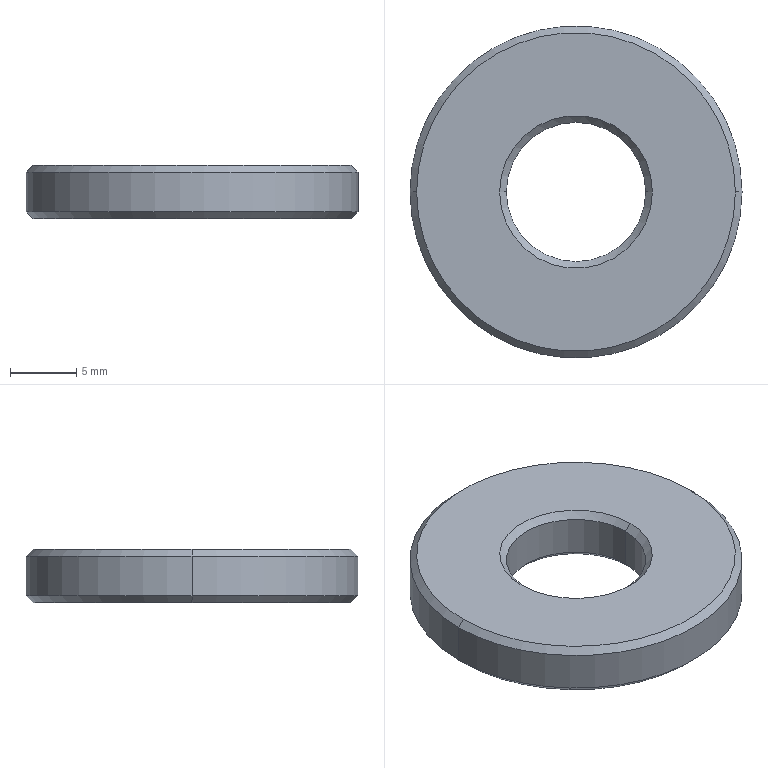Part | STEP file | PN_0101 Mount electronic clip clamp screw | 1 solid | 14 faces | box 25 x 25 x 4 mm | volume 1589 mm3 | cone 8 | cylinder 4 | plane 2 | commonest cylinder face diameters 10.5 x2 25 x2
STEP:
#1=CARTESIAN_POINT('',(0.,0.,0.));
#2=DIRECTION('',(0.,0.,1.));
#3=DIRECTION('',(1.,0.,0.));
#4=AXIS2_PLACEMENT_3D('',#1,#2,#3);
#5=CARTESIAN_POINT('',(12.,0.,4.));
#6=VERTEX_POINT('',#5);
#7=CARTESIAN_POINT('',(-12.,0.,4.));
#8=VERTEX_POINT('',#7);
#9=CARTESIAN_POINT('',(0.,0.,4.));
#10=DIRECTION('',(0.,0.,1.));
#11=DIRECTION('',(1.,0.,0.));
#12=AXIS2_PLACEMENT_3D('',#9,#10,#11);
#13=CIRCLE('',#12,12.);
#14=CARTESIAN_POINT('',(0.,0.,4.));
#15=DIRECTION('',(0.,0.,-1.));
#16=DIRECTION('',(-1.,0.,0.));
#17=AXIS2_PLACEMENT_3D('',#14,#15,#16);
#18=CONICAL_SURFACE('',#17,12.,0.7854);
#19=CARTESIAN_POINT('',(3.142,0.));
#20=DIRECTION('',(-1.,0.));
#21=VECTOR('',#20,1.);
#22=LINE('',#19,#21);
#23=(GEOMETRIC_REPRESENTATION_CONTEXT(2)PARAMETRIC_REPRESENTATION_CONTEXT()REPRESENTATION_CONTEXT('',''));
#24=DEFINITIONAL_REPRESENTATION('',(#22),#23);
#25=PCURVE('',#18,#24);
#26=CARTESIAN_POINT('',(0.,0.,4.));
#27=DIRECTION('',(0.,0.,1.));
#28=DIRECTION('',(1.,0.,0.));
#29=AXIS2_PLACEMENT_3D('',#26,#27,#28);
#30=PLANE('',#29);
#31=CARTESIAN_POINT('',(0.,0.));
#32=DIRECTION('',(1.,0.));
#33=AXIS2_PLACEMENT_2D('',#31,#32);
#34=CIRCLE('',#33,12.);
#35=(GEOMETRIC_REPRESENTATION_CONTEXT(2)PARAMETRIC_REPRESENTATION_CONTEXT()REPRESENTATION_CONTEXT('',''));
#36=DEFINITIONAL_REPRESENTATION('',(#34),#35);
#37=PCURVE('',#30,#36);
#38=SURFACE_CURVE('',#13,(#25,#37),.PCURVE_S1.);
#39=EDGE_CURVE('',#6,#8,#38,.T.);
#40=ORIENTED_EDGE('',*,*,#39,.F.);
#41=CARTESIAN_POINT('',(12.5,0.,3.5));
#42=VERTEX_POINT('',#41);
#43=CARTESIAN_POINT('',(12.,0.,4.));
#44=DIRECTION('',(0.7071,0.,-0.7071));
#45=VECTOR('',#44,1.);
#46=LINE('',#43,#45);
#47=CARTESIAN_POINT('',(3.142,0.));
#48=DIRECTION('',(0.,1.));
#49=VECTOR('',#48,1.);
#50=LINE('',#47,#49);
#51=(GEOMETRIC_REPRESENTATION_CONTEXT(2)PARAMETRIC_REPRESENTATION_CONTEXT()REPRESENTATION_CONTEXT('',''));
#52=DEFINITIONAL_REPRESENTATION('',(#50),#51);
#53=PCURVE('',#18,#52);
#54=CARTESIAN_POINT('',(0.,0.,4.));
#55=DIRECTION('',(0.,0.,-1.));
#56=DIRECTION('',(-1.,0.,0.));
#57=AXIS2_PLACEMENT_3D('',#54,#55,#56);
#58=CONICAL_SURFACE('',#57,12.,0.7854);
#59=CARTESIAN_POINT('',(3.142,0.));
#60=DIRECTION('',(0.,1.));
#61=VECTOR('',#60,1.);
#62=LINE('',#59,#61);
#63=(GEOMETRIC_REPRESENTATION_CONTEXT(2)PARAMETRIC_REPRESENTATION_CONTEXT()REPRESENTATION_CONTEXT('',''));
#64=DEFINITIONAL_REPRESENTATION('',(#62),#63);
#65=PCURVE('',#58,#64);
#66=SURFACE_CURVE('',#46,(#53,#65),.PCURVE_S1.);
#67=EDGE_CURVE('',#6,#42,#66,.T.);
#68=ORIENTED_EDGE('',*,*,#67,.T.);
#69=CARTESIAN_POINT('',(-12.5,0.,3.5));
#70=VERTEX_POINT('',#69);
#71=CARTESIAN_POINT('',(0.,0.,3.5));
#72=DIRECTION('',(0.,0.,-1.));
#73=DIRECTION('',(1.,0.,0.));
#74=AXIS2_PLACEMENT_3D('',#71,#72,#73);
#75=CIRCLE('',#74,12.5);
#76=CARTESIAN_POINT('',(-3.142,0.5));
#77=DIRECTION('',(1.,0.));
#78=VECTOR('',#77,1.);
#79=LINE('',#76,#78);
#80=(GEOMETRIC_REPRESENTATION_CONTEXT(2)PARAMETRIC_REPRESENTATION_CONTEXT()REPRESENTATION_CONTEXT('',''));
#81=DEFINITIONAL_REPRESENTATION('',(#79),#80);
#82=PCURVE('',#18,#81);
#83=CARTESIAN_POINT('',(0.,0.,4.));
#84=DIRECTION('',(0.,0.,-1.));
#85=DIRECTION('',(-1.,0.,0.));
#86=AXIS2_PLACEMENT_3D('',#83,#84,#85);
#87=CYLINDRICAL_SURFACE('',#86,12.5);
#88=CARTESIAN_POINT('',(-3.142,0.5));
#89=DIRECTION('',(1.,0.));
#90=VECTOR('',#89,1.);
#91=LINE('',#88,#90);
#92=(GEOMETRIC_REPRESENTATION_CONTEXT(2)PARAMETRIC_REPRESENTATION_CONTEXT()REPRESENTATION_CONTEXT('',''));
#93=DEFINITIONAL_REPRESENTATION('',(#91),#92);
#94=PCURVE('',#87,#93);
#95=SURFACE_CURVE('',#75,(#82,#94),.PCURVE_S1.);
#96=EDGE_CURVE('',#70,#42,#95,.T.);
#97=ORIENTED_EDGE('',*,*,#96,.F.);
#98=CARTESIAN_POINT('',(-12.,0.,4.));
#99=DIRECTION('',(-0.7071,0.,-0.7071));
#100=VECTOR('',#99,1.);
#101=LINE('',#98,#100);
#102=CARTESIAN_POINT('',(0.,0.));
#103=DIRECTION('',(0.,1.));
#104=VECTOR('',#103,1.);
#105=LINE('',#102,#104);
#106=(GEOMETRIC_REPRESENTATION_CONTEXT(2)PARAMETRIC_REPRESENTATION_CONTEXT()REPRESENTATION_CONTEXT('',''));
#107=DEFINITIONAL_REPRESENTATION('',(#105),#106);
#108=PCURVE('',#18,#107);
#109=CARTESIAN_POINT('',(6.283,0.));
#110=DIRECTION('',(0.,1.));
#111=VECTOR('',#110,1.);
#112=LINE('',#109,#111);
#113=(GEOMETRIC_REPRESENTATION_CONTEXT(2)PARAMETRIC_REPRESENTATION_CONTEXT()REPRESENTATION_CONTEXT('',''));
#114=DEFINITIONAL_REPRESENTATION('',(#112),#113);
#115=PCURVE('',#58,#114);
#116=SURFACE_CURVE('',#101,(#108,#115),.PCURVE_S1.);
#117=EDGE_CURVE('',#8,#70,#116,.T.);
#118=ORIENTED_EDGE('',*,*,#117,.F.);
#119=EDGE_LOOP('',(#40,#68,#97,#118));
#120=FACE_BOUND('',#119,.T.);
#121=ADVANCED_FACE('',(#120),#18,.T.);
#122=CARTESIAN_POINT('',(-12.,0.,0.));
#123=VERTEX_POINT('',#122);
#124=CARTESIAN_POINT('',(12.,0.,0.));
#125=VERTEX_POINT('',#124);
#126=CARTESIAN_POINT('',(0.,0.,0.));
#127=DIRECTION('',(0.,0.,-1.));
#128=DIRECTION('',(1.,0.,0.));
#129=AXIS2_PLACEMENT_3D('',#126,#127,#128);
#130=CIRCLE('',#129,12.);
#131=CARTESIAN_POINT('',(0.,0.,0.5));
#132=DIRECTION('',(0.,0.,1.));
#133=DIRECTION('',(1.,0.,0.));
#134=AXIS2_PLACEMENT_3D('',#131,#132,#133);
#135=CONICAL_SURFACE('',#134,12.5,0.7854);
#136=CARTESIAN_POINT('',(6.283,-0.5));
#137=DIRECTION('',(-1.,0.));
#138=VECTOR('',#137,1.);
#139=LINE('',#136,#138);
#140=(GEOMETRIC_REPRESENTATION_CONTEXT(2)PARAMETRIC_REPRESENTATION_CONTEXT()REPRESENTATION_CONTEXT('',''));
#141=DEFINITIONAL_REPRESENTATION('',(#139),#140);
#142=PCURVE('',#135,#141);
#143=CARTESIAN_POINT('',(0.,0.,0.));
#144=DIRECTION('',(0.,0.,1.));
#145=DIRECTION('',(1.,0.,0.));
#146=AXIS2_PLACEMENT_3D('',#143,#144,#145);
#147=PLANE('',#146);
#148=CARTESIAN_POINT('',(12.,0.));
#149=CARTESIAN_POINT('',(12.,-20.785));
#150=CARTESIAN_POINT('',(-6.,-10.392));
#151=CARTESIAN_POINT('',(-24.,0.));
#152=CARTESIAN_POINT('',(-6.,10.392));
#153=CARTESIAN_POINT('',(12.,20.785));
#154=CARTESIAN_POINT('',(12.,0.));
#155=(BOUNDED_CURVE()B_SPLINE_CURVE(2,(#148,#149,#150,#151,#152,#153,#154),.UNSPECIFIED.,.T.,.F.)B_SPLINE_CURVE_WITH_KNOTS((1,2,2,2,2,1),(-2.094,0.,2.094,4.189,6.283,8.378),.UNSPECIFIED.)CURVE()GEOMETRIC_REPRESENTATION_ITEM()RATIONAL_B_SPLINE_CURVE((1.,0.5,1.,0.5,1.,0.5,1.))REPRESENTATION_ITEM(''));
#156=(GEOMETRIC_REPRESENTATION_CONTEXT(2)PARAMETRIC_REPRESENTATION_CONTEXT()REPRESENTATION_CONTEXT('',''));
#157=DEFINITIONAL_REPRESENTATION('',(#155),#156);
#158=PCURVE('',#147,#157);
#159=SURFACE_CURVE('',#130,(#142,#158),.PCURVE_S1.);
#160=EDGE_CURVE('',#123,#125,#159,.T.);
#161=ORIENTED_EDGE('',*,*,#160,.F.);
#162=CARTESIAN_POINT('',(-12.5,0.,0.5));
#163=VERTEX_POINT('',#162);
#164=CARTESIAN_POINT('',(-12.5,0.,0.5));
#165=DIRECTION('',(-0.7071,0.,0.7071));
#166=VECTOR('',#165,1.);
#167=LINE('',#164,#166);
#168=CARTESIAN_POINT('',(3.142,0.));
#169=DIRECTION('',(0.,1.));
#170=VECTOR('',#169,1.);
#171=LINE('',#168,#170);
#172=(GEOMETRIC_REPRESENTATION_CONTEXT(2)PARAMETRIC_REPRESENTATION_CONTEXT()REPRESENTATION_CONTEXT('',''));
#173=DEFINITIONAL_REPRESENTATION('',(#171),#172);
#174=PCURVE('',#135,#173);
#175=CARTESIAN_POINT('',(0.,0.,0.5));
#176=DIRECTION('',(0.,0.,1.));
#177=DIRECTION('',(1.,0.,0.));
#178=AXIS2_PLACEMENT_3D('',#175,#176,#177);
#179=CONICAL_SURFACE('',#178,12.5,0.7854);
#180=CARTESIAN_POINT('',(3.142,0.));
#181=DIRECTION('',(0.,1.));
#182=VECTOR('',#181,1.);
#183=LINE('',#180,#182);
#184=(GEOMETRIC_REPRESENTATION_CONTEXT(2)PARAMETRIC_REPRESENTATION_CONTEXT()REPRESENTATION_CONTEXT('',''));
#185=DEFINITIONAL_REPRESENTATION('',(#183),#184);
#186=PCURVE('',#179,#185);
#187=SURFACE_CURVE('',#167,(#174,#186),.PCURVE_S1.);
#188=EDGE_CURVE('',#123,#163,#187,.T.);
#189=ORIENTED_EDGE('',*,*,#188,.T.);
#190=CARTESIAN_POINT('',(12.5,0.,0.5));
#191=VERTEX_POINT('',#190);
#192=CARTESIAN_POINT('',(0.,0.,0.5));
#193=DIRECTION('',(0.,0.,1.));
#194=DIRECTION('',(1.,0.,0.));
#195=AXIS2_PLACEMENT_3D('',#192,#193,#194);
#196=CIRCLE('',#195,12.5);
#197=CARTESIAN_POINT('',(0.,0.));
#198=DIRECTION('',(1.,0.));
#199=VECTOR('',#198,1.);
#200=LINE('',#197,#199);
#201=(GEOMETRIC_REPRESENTATION_CONTEXT(2)PARAMETRIC_REPRESENTATION_CONTEXT()REPRESENTATION_CONTEXT('',''));
#202=DEFINITIONAL_REPRESENTATION('',(#200),#201);
#203=PCURVE('',#135,#202);
#204=CARTESIAN_POINT('',(3.142,3.5));
#205=DIRECTION('',(-1.,0.));
#206=VECTOR('',#205,1.);
#207=LINE('',#204,#206);
#208=(GEOMETRIC_REPRESENTATION_CONTEXT(2)PARAMETRIC_REPRESENTATION_CONTEXT()REPRESENTATION_CONTEXT('',''));
#209=DEFINITIONAL_REPRESENTATION('',(#207),#208);
#210=PCURVE('',#87,#209);
#211=SURFACE_CURVE('',#196,(#203,#210),.PCURVE_S1.);
#212=EDGE_CURVE('',#191,#163,#211,.T.);
#213=ORIENTED_EDGE('',*,*,#212,.F.);
#214=CARTESIAN_POINT('',(12.5,0.,0.5));
#215=DIRECTION('',(0.7071,0.,0.7071));
#216=VECTOR('',#215,1.);
#217=LINE('',#214,#216);
#218=CARTESIAN_POINT('',(0.,0.));
#219=DIRECTION('',(0.,1.));
#220=VECTOR('',#219,1.);
#221=LINE('',#218,#220);
#222=(GEOMETRIC_REPRESENTATION_CONTEXT(2)PARAMETRIC_REPRESENTATION_CONTEXT()REPRESENTATION_CONTEXT('',''));
#223=DEFINITIONAL_REPRESENTATION('',(#221),#222);
#224=PCURVE('',#135,#223);
#225=CARTESIAN_POINT('',(6.283,0.));
#226=DIRECTION('',(0.,1.));
#227=VECTOR('',#226,1.);
#228=LINE('',#225,#227);
#229=(GEOMETRIC_REPRESENTATION_CONTEXT(2)PARAMETRIC_REPRESENTATION_CONTEXT()REPRESENTATION_CONTEXT('',''));
#230=DEFINITIONAL_REPRESENTATION('',(#228),#229);
#231=PCURVE('',#179,#230);
#232=SURFACE_CURVE('',#217,(#224,#231),.PCURVE_S1.);
#233=EDGE_CURVE('',#125,#191,#232,.T.);
#234=ORIENTED_EDGE('',*,*,#233,.F.);
#235=EDGE_LOOP('',(#161,#189,#213,#234));
#236=FACE_BOUND('',#235,.T.);
#237=ADVANCED_FACE('',(#236),#135,.T.);
#238=CARTESIAN_POINT('',(-5.25,0.,0.5));
#239=VERTEX_POINT('',#238);
#240=CARTESIAN_POINT('',(-5.75,0.,0.));
#241=VERTEX_POINT('',#240);
#242=CARTESIAN_POINT('',(-5.75,0.,0.));
#243=DIRECTION('',(-0.7071,0.,-0.7071));
#244=VECTOR('',#243,1.);
#245=LINE('',#242,#244);
#246=CARTESIAN_POINT('',(0.,0.,0.));
#247=DIRECTION('',(0.,0.,-1.));
#248=DIRECTION('',(-1.,0.,0.));
#249=AXIS2_PLACEMENT_3D('',#246,#247,#248);
#250=CONICAL_SURFACE('',#249,5.75,0.7854);
#251=CARTESIAN_POINT('',(6.283,0.));
#252=DIRECTION('',(0.,1.));
#253=VECTOR('',#252,1.);
#254=LINE('',#251,#253);
#255=(GEOMETRIC_REPRESENTATION_CONTEXT(2)PARAMETRIC_REPRESENTATION_CONTEXT()REPRESENTATION_CONTEXT('',''));
#256=DEFINITIONAL_REPRESENTATION('',(#254),#255);
#257=PCURVE('',#250,#256);
#258=CARTESIAN_POINT('',(0.,0.,0.));
#259=DIRECTION('',(0.,0.,-1.));
#260=DIRECTION('',(-1.,0.,0.));
#261=AXIS2_PLACEMENT_3D('',#258,#259,#260);
#262=CONICAL_SURFACE('',#261,5.75,0.7854);
#263=CARTESIAN_POINT('',(0.,0.));
#264=DIRECTION('',(0.,1.));
#265=VECTOR('',#264,1.);
#266=LINE('',#263,#265);
#267=(GEOMETRIC_REPRESENTATION_CONTEXT(2)PARAMETRIC_REPRESENTATION_CONTEXT()REPRESENTATION_CONTEXT('',''));
#268=DEFINITIONAL_REPRESENTATION('',(#266),#267);
#269=PCURVE('',#262,#268);
#270=SURFACE_CURVE('',#245,(#257,#269),.PCURVE_S1.);
#271=EDGE_CURVE('',#239,#241,#270,.T.);
#272=ORIENTED_EDGE('',*,*,#271,.T.);
#273=CARTESIAN_POINT('',(5.75,0.,0.));
#274=VERTEX_POINT('',#273);
#275=CARTESIAN_POINT('',(0.,0.,0.));
#276=DIRECTION('',(0.,0.,1.));
#277=DIRECTION('',(1.,0.,0.));
#278=AXIS2_PLACEMENT_3D('',#275,#276,#277);
#279=CIRCLE('',#278,5.75);
#280=CARTESIAN_POINT('',(9.425,0.));
#281=DIRECTION('',(-1.,0.));
#282=VECTOR('',#281,1.);
#283=LINE('',#280,#282);
#284=(GEOMETRIC_REPRESENTATION_CONTEXT(2)PARAMETRIC_REPRESENTATION_CONTEXT()REPRESENTATION_CONTEXT('',''));
#285=DEFINITIONAL_REPRESENTATION('',(#283),#284);
#286=PCURVE('',#250,#285);
#287=CARTESIAN_POINT('',(0.,0.));
#288=DIRECTION('',(1.,0.));
#289=AXIS2_PLACEMENT_2D('',#287,#288);
#290=CIRCLE('',#289,5.75);
#291=(GEOMETRIC_REPRESENTATION_CONTEXT(2)PARAMETRIC_REPRESENTATION_CONTEXT()REPRESENTATION_CONTEXT('',''));
#292=DEFINITIONAL_REPRESENTATION('',(#290),#291);
#293=PCURVE('',#147,#292);
#294=SURFACE_CURVE('',#279,(#286,#293),.PCURVE_S1.);
#295=EDGE_CURVE('',#241,#274,#294,.T.);
#296=ORIENTED_EDGE('',*,*,#295,.T.);
#297=CARTESIAN_POINT('',(5.25,0.,0.5));
#298=VERTEX_POINT('',#297);
#299=CARTESIAN_POINT('',(5.75,0.,0.));
#300=DIRECTION('',(0.7071,0.,-0.7071));
#301=VECTOR('',#300,1.);
#302=LINE('',#299,#301);
#303=CARTESIAN_POINT('',(3.142,0.));
#304=DIRECTION('',(0.,1.));
#305=VECTOR('',#304,1.);
#306=LINE('',#303,#305);
#307=(GEOMETRIC_REPRESENTATION_CONTEXT(2)PARAMETRIC_REPRESENTATION_CONTEXT()REPRESENTATION_CONTEXT('',''));
#308=DEFINITIONAL_REPRESENTATION('',(#306),#307);
#309=PCURVE('',#250,#308);
#310=CARTESIAN_POINT('',(3.142,0.));
#311=DIRECTION('',(0.,1.));
#312=VECTOR('',#311,1.);
#313=LINE('',#310,#312);
#314=(GEOMETRIC_REPRESENTATION_CONTEXT(2)PARAMETRIC_REPRESENTATION_CONTEXT()REPRESENTATION_CONTEXT('',''));
#315=DEFINITIONAL_REPRESENTATION('',(#313),#314);
#316=PCURVE('',#262,#315);
#317=SURFACE_CURVE('',#302,(#309,#316),.PCURVE_S1.);
#318=EDGE_CURVE('',#298,#274,#317,.T.);
#319=ORIENTED_EDGE('',*,*,#318,.F.);
#320=CARTESIAN_POINT('',(0.,0.,0.5));
#321=DIRECTION('',(0.,0.,-1.));
#322=DIRECTION('',(1.,0.,0.));
#323=AXIS2_PLACEMENT_3D('',#320,#321,#322);
#324=CIRCLE('',#323,5.25);
#325=CARTESIAN_POINT('',(3.142,-0.5));
#326=DIRECTION('',(1.,0.));
#327=VECTOR('',#326,1.);
#328=LINE('',#325,#327);
#329=(GEOMETRIC_REPRESENTATION_CONTEXT(2)PARAMETRIC_REPRESENTATION_CONTEXT()REPRESENTATION_CONTEXT('',''));
#330=DEFINITIONAL_REPRESENTATION('',(#328),#329);
#331=PCURVE('',#250,#330);
#332=CARTESIAN_POINT('',(0.,0.,0.));
#333=DIRECTION('',(0.,0.,1.));
#334=DIRECTION('',(1.,0.,0.));
#335=AXIS2_PLACEMENT_3D('',#332,#333,#334);
#336=CYLINDRICAL_SURFACE('',#335,5.25);
#337=CARTESIAN_POINT('',(6.283,0.5));
#338=DIRECTION('',(-1.,0.));
#339=VECTOR('',#338,1.);
#340=LINE('',#337,#339);
#341=(GEOMETRIC_REPRESENTATION_CONTEXT(2)PARAMETRIC_REPRESENTATION_CONTEXT()REPRESENTATION_CONTEXT('',''));
#342=DEFINITIONAL_REPRESENTATION('',(#340),#341);
#343=PCURVE('',#336,#342);
#344=SURFACE_CURVE('',#324,(#331,#343),.PCURVE_S1.);
#345=EDGE_CURVE('',#298,#239,#344,.T.);
#346=ORIENTED_EDGE('',*,*,#345,.T.);
#347=EDGE_LOOP('',(#272,#296,#319,#346));
#348=FACE_BOUND('',#347,.F.);
#349=ADVANCED_FACE('',(#348),#250,.F.);
#350=CARTESIAN_POINT('',(5.25,0.,3.5));
#351=VERTEX_POINT('',#350);
#352=CARTESIAN_POINT('',(5.75,0.,4.));
#353=VERTEX_POINT('',#352);
#354=CARTESIAN_POINT('',(5.25,0.,3.5));
#355=DIRECTION('',(0.7071,0.,0.7071));
#356=VECTOR('',#355,1.);
#357=LINE('',#354,#356);
#358=CARTESIAN_POINT('',(0.,0.,3.5));
#359=DIRECTION('',(0.,0.,1.));
#360=DIRECTION('',(1.,0.,0.));
#361=AXIS2_PLACEMENT_3D('',#358,#359,#360);
#362=CONICAL_SURFACE('',#361,5.25,0.7854);
#363=CARTESIAN_POINT('',(6.283,0.));
#364=DIRECTION('',(0.,1.));
#365=VECTOR('',#364,1.);
#366=LINE('',#363,#365);
#367=(GEOMETRIC_REPRESENTATION_CONTEXT(2)PARAMETRIC_REPRESENTATION_CONTEXT()REPRESENTATION_CONTEXT('',''));
#368=DEFINITIONAL_REPRESENTATION('',(#366),#367);
#369=PCURVE('',#362,#368);
#370=CARTESIAN_POINT('',(0.,0.,3.5));
#371=DIRECTION('',(0.,0.,1.));
#372=DIRECTION('',(1.,0.,0.));
#373=AXIS2_PLACEMENT_3D('',#370,#371,#372);
#374=CONICAL_SURFACE('',#373,5.25,0.7854);
#375=CARTESIAN_POINT('',(0.,0.));
#376=DIRECTION('',(0.,1.));
#377=VECTOR('',#376,1.);
#378=LINE('',#375,#377);
#379=(GEOMETRIC_REPRESENTATION_CONTEXT(2)PARAMETRIC_REPRESENTATION_CONTEXT()REPRESENTATION_CONTEXT('',''));
#380=DEFINITIONAL_REPRESENTATION('',(#378),#379);
#381=PCURVE('',#374,#380);
#382=SURFACE_CURVE('',#357,(#369,#381),.PCURVE_S1.);
#383=EDGE_CURVE('',#351,#353,#382,.T.);
#384=ORIENTED_EDGE('',*,*,#383,.T.);
#385=CARTESIAN_POINT('',(-5.75,0.,4.));
#386=VERTEX_POINT('',#385);
#387=CARTESIAN_POINT('',(0.,0.,4.));
#388=DIRECTION('',(0.,0.,-1.));
#389=DIRECTION('',(1.,0.,0.));
#390=AXIS2_PLACEMENT_3D('',#387,#388,#389);
#391=CIRCLE('',#390,5.75);
#392=CARTESIAN_POINT('',(6.283,0.5));
#393=DIRECTION('',(-1.,0.));
#394=VECTOR('',#393,1.);
#395=LINE('',#392,#394);
#396=(GEOMETRIC_REPRESENTATION_CONTEXT(2)PARAMETRIC_REPRESENTATION_CONTEXT()REPRESENTATION_CONTEXT('',''));
#397=DEFINITIONAL_REPRESENTATION('',(#395),#396);
#398=PCURVE('',#362,#397);
#399=CARTESIAN_POINT('',(5.75,0.));
#400=CARTESIAN_POINT('',(5.75,-9.959));
#401=CARTESIAN_POINT('',(-2.875,-4.98));
#402=CARTESIAN_POINT('',(-11.5,0.));
#403=CARTESIAN_POINT('',(-2.875,4.98));
#404=CARTESIAN_POINT('',(5.75,9.959));
#405=CARTESIAN_POINT('',(5.75,0.));
#406=(BOUNDED_CURVE()B_SPLINE_CURVE(2,(#399,#400,#401,#402,#403,#404,#405),.UNSPECIFIED.,.T.,.F.)B_SPLINE_CURVE_WITH_KNOTS((1,2,2,2,2,1),(-2.094,0.,2.094,4.189,6.283,8.378),.UNSPECIFIED.)CURVE()GEOMETRIC_REPRESENTATION_ITEM()RATIONAL_B_SPLINE_CURVE((1.,0.5,1.,0.5,1.,0.5,1.))REPRESENTATION_ITEM(''));
#407=(GEOMETRIC_REPRESENTATION_CONTEXT(2)PARAMETRIC_REPRESENTATION_CONTEXT()REPRESENTATION_CONTEXT('',''));
#408=DEFINITIONAL_REPRESENTATION('',(#406),#407);
#409=PCURVE('',#30,#408);
#410=SURFACE_CURVE('',#391,(#398,#409),.PCURVE_S1.);
#411=EDGE_CURVE('',#353,#386,#410,.T.);
#412=ORIENTED_EDGE('',*,*,#411,.T.);
#413=CARTESIAN_POINT('',(-5.25,0.,3.5));
#414=VERTEX_POINT('',#413);
#415=CARTESIAN_POINT('',(-5.25,0.,3.5));
#416=DIRECTION('',(-0.7071,0.,0.7071));
#417=VECTOR('',#416,1.);
#418=LINE('',#415,#417);
#419=CARTESIAN_POINT('',(3.142,0.));
#420=DIRECTION('',(0.,1.));
#421=VECTOR('',#420,1.);
#422=LINE('',#419,#421);
#423=(GEOMETRIC_REPRESENTATION_CONTEXT(2)PARAMETRIC_REPRESENTATION_CONTEXT()REPRESENTATION_CONTEXT('',''));
#424=DEFINITIONAL_REPRESENTATION('',(#422),#423);
#425=PCURVE('',#362,#424);
#426=CARTESIAN_POINT('',(3.142,0.));
#427=DIRECTION('',(0.,1.));
#428=VECTOR('',#427,1.);
#429=LINE('',#426,#428);
#430=(GEOMETRIC_REPRESENTATION_CONTEXT(2)PARAMETRIC_REPRESENTATION_CONTEXT()REPRESENTATION_CONTEXT('',''));
#431=DEFINITIONAL_REPRESENTATION('',(#429),#430);
#432=PCURVE('',#374,#431);
#433=SURFACE_CURVE('',#418,(#425,#432),.PCURVE_S1.);
#434=EDGE_CURVE('',#414,#386,#433,.T.);
#435=ORIENTED_EDGE('',*,*,#434,.F.);
#436=CARTESIAN_POINT('',(0.,0.,3.5));
#437=DIRECTION('',(0.,0.,1.));
#438=DIRECTION('',(1.,0.,0.));
#439=AXIS2_PLACEMENT_3D('',#436,#437,#438);
#440=CIRCLE('',#439,5.25);
#441=CARTESIAN_POINT('',(0.,0.));
#442=DIRECTION('',(1.,0.));
#443=VECTOR('',#442,1.);
#444=LINE('',#441,#443);
#445=(GEOMETRIC_REPRESENTATION_CONTEXT(2)PARAMETRIC_REPRESENTATION_CONTEXT()REPRESENTATION_CONTEXT('',''));
#446=DEFINITIONAL_REPRESENTATION('',(#444),#445);
#447=PCURVE('',#362,#446);
#448=CARTESIAN_POINT('',(0.,3.5));
#449=DIRECTION('',(1.,0.));
#450=VECTOR('',#449,1.);
#451=LINE('',#448,#450);
#452=(GEOMETRIC_REPRESENTATION_CONTEXT(2)PARAMETRIC_REPRESENTATION_CONTEXT()REPRESENTATION_CONTEXT('',''));
#453=DEFINITIONAL_REPRESENTATION('',(#451),#452);
#454=PCURVE('',#336,#453);
#455=SURFACE_CURVE('',#440,(#447,#454),.PCURVE_S1.);
#456=EDGE_CURVE('',#414,#351,#455,.T.);
#457=ORIENTED_EDGE('',*,*,#456,.T.);
#458=EDGE_LOOP('',(#384,#412,#435,#457));
#459=FACE_BOUND('',#458,.F.);
#460=ADVANCED_FACE('',(#459),#362,.F.);
#461=CARTESIAN_POINT('',(5.25,0.,0.));
#462=DIRECTION('',(0.,0.,1.));
#463=VECTOR('',#462,1.);
#464=LINE('',#461,#463);
#465=CARTESIAN_POINT('',(6.283,0.));
#466=DIRECTION('',(0.,1.));
#467=VECTOR('',#466,1.);
#468=LINE('',#465,#467);
#469=(GEOMETRIC_REPRESENTATION_CONTEXT(2)PARAMETRIC_REPRESENTATION_CONTEXT()REPRESENTATION_CONTEXT('',''));
#470=DEFINITIONAL_REPRESENTATION('',(#468),#469);
#471=PCURVE('',#336,#470);
#472=CARTESIAN_POINT('',(0.,0.,0.));
#473=DIRECTION('',(0.,0.,1.));
#474=DIRECTION('',(1.,0.,0.));
#475=AXIS2_PLACEMENT_3D('',#472,#473,#474);
#476=CYLINDRICAL_SURFACE('',#475,5.25);
#477=CARTESIAN_POINT('',(0.,0.));
#478=DIRECTION('',(0.,1.));
#479=VECTOR('',#478,1.);
#480=LINE('',#477,#479);
#481=(GEOMETRIC_REPRESENTATION_CONTEXT(2)PARAMETRIC_REPRESENTATION_CONTEXT()REPRESENTATION_CONTEXT('',''));
#482=DEFINITIONAL_REPRESENTATION('',(#480),#481);
#483=PCURVE('',#476,#482);
#484=SURFACE_CURVE('',#464,(#471,#483),.PCURVE_S1.);
#485=EDGE_CURVE('',#298,#351,#484,.T.);
#486=ORIENTED_EDGE('',*,*,#485,.T.);
#487=ORIENTED_EDGE('',*,*,#456,.F.);
#488=CARTESIAN_POINT('',(-5.25,0.,0.));
#489=DIRECTION('',(0.,0.,1.));
#490=VECTOR('',#489,1.);
#491=LINE('',#488,#490);
#492=CARTESIAN_POINT('',(3.142,0.));
#493=DIRECTION('',(0.,1.));
#494=VECTOR('',#493,1.);
#495=LINE('',#492,#494);
#496=(GEOMETRIC_REPRESENTATION_CONTEXT(2)PARAMETRIC_REPRESENTATION_CONTEXT()REPRESENTATION_CONTEXT('',''));
#497=DEFINITIONAL_REPRESENTATION('',(#495),#496);
#498=PCURVE('',#336,#497);
#499=CARTESIAN_POINT('',(3.142,0.));
#500=DIRECTION('',(0.,1.));
#501=VECTOR('',#500,1.);
#502=LINE('',#499,#501);
#503=(GEOMETRIC_REPRESENTATION_CONTEXT(2)PARAMETRIC_REPRESENTATION_CONTEXT()REPRESENTATION_CONTEXT('',''));
#504=DEFINITIONAL_REPRESENTATION('',(#502),#503);
#505=PCURVE('',#476,#504);
#506=SURFACE_CURVE('',#491,(#498,#505),.PCURVE_S1.);
#507=EDGE_CURVE('',#239,#414,#506,.T.);
#508=ORIENTED_EDGE('',*,*,#507,.F.);
#509=ORIENTED_EDGE('',*,*,#345,.F.);
#510=EDGE_LOOP('',(#486,#487,#508,#509));
#511=FACE_BOUND('',#510,.F.);
#512=ADVANCED_FACE('',(#511),#336,.F.);
#513=ORIENTED_EDGE('',*,*,#96,.T.);
#514=CARTESIAN_POINT('',(12.5,0.,4.));
#515=DIRECTION('',(0.,0.,-1.));
#516=VECTOR('',#515,1.);
#517=LINE('',#514,#516);
#518=CARTESIAN_POINT('',(3.142,0.));
#519=DIRECTION('',(0.,1.));
#520=VECTOR('',#519,1.);
#521=LINE('',#518,#520);
#522=(GEOMETRIC_REPRESENTATION_CONTEXT(2)PARAMETRIC_REPRESENTATION_CONTEXT()REPRESENTATION_CONTEXT('',''));
#523=DEFINITIONAL_REPRESENTATION('',(#521),#522);
#524=PCURVE('',#87,#523);
#525=CARTESIAN_POINT('',(0.,0.,4.));
#526=DIRECTION('',(0.,0.,-1.));
#527=DIRECTION('',(-1.,0.,0.));
#528=AXIS2_PLACEMENT_3D('',#525,#526,#527);
#529=CYLINDRICAL_SURFACE('',#528,12.5);
#530=CARTESIAN_POINT('',(3.142,0.));
#531=DIRECTION('',(0.,1.));
#532=VECTOR('',#531,1.);
#533=LINE('',#530,#532);
#534=(GEOMETRIC_REPRESENTATION_CONTEXT(2)PARAMETRIC_REPRESENTATION_CONTEXT()REPRESENTATION_CONTEXT('',''));
#535=DEFINITIONAL_REPRESENTATION('',(#533),#534);
#536=PCURVE('',#529,#535);
#537=SURFACE_CURVE('',#517,(#524,#536),.PCURVE_S1.);
#538=EDGE_CURVE('',#42,#191,#537,.T.);
#539=ORIENTED_EDGE('',*,*,#538,.T.);
#540=ORIENTED_EDGE('',*,*,#212,.T.);
#541=CARTESIAN_POINT('',(-12.5,0.,4.));
#542=DIRECTION('',(0.,0.,-1.));
#543=VECTOR('',#542,1.);
#544=LINE('',#541,#543);
#545=CARTESIAN_POINT('',(0.,0.));
#546=DIRECTION('',(0.,1.));
#547=VECTOR('',#546,1.);
#548=LINE('',#545,#547);
#549=(GEOMETRIC_REPRESENTATION_CONTEXT(2)PARAMETRIC_REPRESENTATION_CONTEXT()REPRESENTATION_CONTEXT('',''));
#550=DEFINITIONAL_REPRESENTATION('',(#548),#549);
#551=PCURVE('',#87,#550);
#552=CARTESIAN_POINT('',(6.283,0.));
#553=DIRECTION('',(0.,1.));
#554=VECTOR('',#553,1.);
#555=LINE('',#552,#554);
#556=(GEOMETRIC_REPRESENTATION_CONTEXT(2)PARAMETRIC_REPRESENTATION_CONTEXT()REPRESENTATION_CONTEXT('',''));
#557=DEFINITIONAL_REPRESENTATION('',(#555),#556);
#558=PCURVE('',#529,#557);
#559=SURFACE_CURVE('',#544,(#551,#558),.PCURVE_S1.);
#560=EDGE_CURVE('',#70,#163,#559,.T.);
#561=ORIENTED_EDGE('',*,*,#560,.F.);
#562=EDGE_LOOP('',(#513,#539,#540,#561));
#563=FACE_BOUND('',#562,.T.);
#564=ADVANCED_FACE('',(#563),#87,.T.);
#565=ORIENTED_EDGE('',*,*,#538,.F.);
#566=CARTESIAN_POINT('',(0.,0.,3.5));
#567=DIRECTION('',(0.,0.,-1.));
#568=DIRECTION('',(1.,0.,0.));
#569=AXIS2_PLACEMENT_3D('',#566,#567,#568);
#570=CIRCLE('',#569,12.5);
#571=CARTESIAN_POINT('',(3.142,0.5));
#572=DIRECTION('',(1.,0.));
#573=VECTOR('',#572,1.);
#574=LINE('',#571,#573);
#575=(GEOMETRIC_REPRESENTATION_CONTEXT(2)PARAMETRIC_REPRESENTATION_CONTEXT()REPRESENTATION_CONTEXT('',''));
#576=DEFINITIONAL_REPRESENTATION('',(#574),#575);
#577=PCURVE('',#529,#576);
#578=CARTESIAN_POINT('',(3.142,0.5));
#579=DIRECTION('',(1.,0.));
#580=VECTOR('',#579,1.);
#581=LINE('',#578,#580);
#582=(GEOMETRIC_REPRESENTATION_CONTEXT(2)PARAMETRIC_REPRESENTATION_CONTEXT()REPRESENTATION_CONTEXT('',''));
#583=DEFINITIONAL_REPRESENTATION('',(#581),#582);
#584=PCURVE('',#58,#583);
#585=SURFACE_CURVE('',#570,(#577,#584),.PCURVE_S1.);
#586=EDGE_CURVE('',#42,#70,#585,.T.);
#587=ORIENTED_EDGE('',*,*,#586,.T.);
#588=ORIENTED_EDGE('',*,*,#560,.T.);
#589=CARTESIAN_POINT('',(0.,0.,0.5));
#590=DIRECTION('',(0.,0.,1.));
#591=DIRECTION('',(1.,0.,0.));
#592=AXIS2_PLACEMENT_3D('',#589,#590,#591);
#593=CIRCLE('',#592,12.5);
#594=CARTESIAN_POINT('',(9.425,3.5));
#595=DIRECTION('',(-1.,0.));
#596=VECTOR('',#595,1.);
#597=LINE('',#594,#596);
#598=(GEOMETRIC_REPRESENTATION_CONTEXT(2)PARAMETRIC_REPRESENTATION_CONTEXT()REPRESENTATION_CONTEXT('',''));
#599=DEFINITIONAL_REPRESENTATION('',(#597),#598);
#600=PCURVE('',#529,#599);
#601=CARTESIAN_POINT('',(0.,0.));
#602=DIRECTION('',(1.,0.));
#603=VECTOR('',#602,1.);
#604=LINE('',#601,#603);
#605=(GEOMETRIC_REPRESENTATION_CONTEXT(2)PARAMETRIC_REPRESENTATION_CONTEXT()REPRESENTATION_CONTEXT('',''));
#606=DEFINITIONAL_REPRESENTATION('',(#604),#605);
#607=PCURVE('',#179,#606);
#608=SURFACE_CURVE('',#593,(#600,#607),.PCURVE_S1.);
#609=EDGE_CURVE('',#163,#191,#608,.T.);
#610=ORIENTED_EDGE('',*,*,#609,.T.);
#611=EDGE_LOOP('',(#565,#587,#588,#610));
#612=FACE_BOUND('',#611,.T.);
#613=ADVANCED_FACE('',(#612),#529,.T.);
#614=ORIENTED_EDGE('',*,*,#411,.T.);
#615=CARTESIAN_POINT('',(0.,0.,4.));
#616=DIRECTION('',(0.,0.,-1.));
#617=DIRECTION('',(1.,0.,0.));
#618=AXIS2_PLACEMENT_3D('',#615,#616,#617);
#619=CIRCLE('',#618,5.75);
#620=CARTESIAN_POINT('',(5.75,0.));
#621=CARTESIAN_POINT('',(5.75,-9.959));
#622=CARTESIAN_POINT('',(-2.875,-4.98));
#623=CARTESIAN_POINT('',(-11.5,0.));
#624=CARTESIAN_POINT('',(-2.875,4.98));
#625=CARTESIAN_POINT('',(5.75,9.959));
#626=CARTESIAN_POINT('',(5.75,0.));
#627=(BOUNDED_CURVE()B_SPLINE_CURVE(2,(#620,#621,#622,#623,#624,#625,#626),.UNSPECIFIED.,.T.,.F.)B_SPLINE_CURVE_WITH_KNOTS((1,2,2,2,2,1),(-2.094,0.,2.094,4.189,6.283,8.378),.UNSPECIFIED.)CURVE()GEOMETRIC_REPRESENTATION_ITEM()RATIONAL_B_SPLINE_CURVE((1.,0.5,1.,0.5,1.,0.5,1.))REPRESENTATION_ITEM(''));
#628=(GEOMETRIC_REPRESENTATION_CONTEXT(2)PARAMETRIC_REPRESENTATION_CONTEXT()REPRESENTATION_CONTEXT('',''));
#629=DEFINITIONAL_REPRESENTATION('',(#627),#628);
#630=PCURVE('',#30,#629);
#631=CARTESIAN_POINT('',(6.283,0.5));
#632=DIRECTION('',(-1.,0.));
#633=VECTOR('',#632,1.);
#634=LINE('',#631,#633);
#635=(GEOMETRIC_REPRESENTATION_CONTEXT(2)PARAMETRIC_REPRESENTATION_CONTEXT()REPRESENTATION_CONTEXT('',''));
#636=DEFINITIONAL_REPRESENTATION('',(#634),#635);
#637=PCURVE('',#374,#636);
#638=SURFACE_CURVE('',#619,(#630,#637),.PCURVE_S1.);
#639=EDGE_CURVE('',#386,#353,#638,.T.);
#640=ORIENTED_EDGE('',*,*,#639,.T.);
#641=EDGE_LOOP('',(#614,#640));
#642=FACE_BOUND('',#641,.T.);
#643=CARTESIAN_POINT('',(0.,0.,4.));
#644=DIRECTION('',(0.,0.,1.));
#645=DIRECTION('',(1.,0.,0.));
#646=AXIS2_PLACEMENT_3D('',#643,#644,#645);
#647=CIRCLE('',#646,12.);
#648=CARTESIAN_POINT('',(0.,0.));
#649=DIRECTION('',(1.,0.));
#650=AXIS2_PLACEMENT_2D('',#648,#649);
#651=CIRCLE('',#650,12.);
#652=(GEOMETRIC_REPRESENTATION_CONTEXT(2)PARAMETRIC_REPRESENTATION_CONTEXT()REPRESENTATION_CONTEXT('',''));
#653=DEFINITIONAL_REPRESENTATION('',(#651),#652);
#654=PCURVE('',#30,#653);
#655=CARTESIAN_POINT('',(9.425,0.));
#656=DIRECTION('',(-1.,0.));
#657=VECTOR('',#656,1.);
#658=LINE('',#655,#657);
#659=(GEOMETRIC_REPRESENTATION_CONTEXT(2)PARAMETRIC_REPRESENTATION_CONTEXT()REPRESENTATION_CONTEXT('',''));
#660=DEFINITIONAL_REPRESENTATION('',(#658),#659);
#661=PCURVE('',#58,#660);
#662=SURFACE_CURVE('',#647,(#654,#661),.PCURVE_S1.);
#663=EDGE_CURVE('',#8,#6,#662,.T.);
#664=ORIENTED_EDGE('',*,*,#663,.T.);
#665=ORIENTED_EDGE('',*,*,#39,.T.);
#666=EDGE_LOOP('',(#664,#665));
#667=FACE_BOUND('',#666,.T.);
#668=ADVANCED_FACE('',(#642,#667),#30,.T.);
#669=ORIENTED_EDGE('',*,*,#295,.T.);
#670=CARTESIAN_POINT('',(0.,0.,0.));
#671=DIRECTION('',(0.,0.,1.));
#672=DIRECTION('',(1.,0.,0.));
#673=AXIS2_PLACEMENT_3D('',#670,#671,#672);
#674=CIRCLE('',#673,5.75);
#675=CARTESIAN_POINT('',(0.,0.));
#676=DIRECTION('',(1.,0.));
#677=AXIS2_PLACEMENT_2D('',#675,#676);
#678=CIRCLE('',#677,5.75);
#679=(GEOMETRIC_REPRESENTATION_CONTEXT(2)PARAMETRIC_REPRESENTATION_CONTEXT()REPRESENTATION_CONTEXT('',''));
#680=DEFINITIONAL_REPRESENTATION('',(#678),#679);
#681=PCURVE('',#147,#680);
#682=CARTESIAN_POINT('',(3.142,0.));
#683=DIRECTION('',(-1.,0.));
#684=VECTOR('',#683,1.);
#685=LINE('',#682,#684);
#686=(GEOMETRIC_REPRESENTATION_CONTEXT(2)PARAMETRIC_REPRESENTATION_CONTEXT()REPRESENTATION_CONTEXT('',''));
#687=DEFINITIONAL_REPRESENTATION('',(#685),#686);
#688=PCURVE('',#262,#687);
#689=SURFACE_CURVE('',#674,(#681,#688),.PCURVE_S1.);
#690=EDGE_CURVE('',#274,#241,#689,.T.);
#691=ORIENTED_EDGE('',*,*,#690,.T.);
#692=EDGE_LOOP('',(#669,#691));
#693=FACE_BOUND('',#692,.T.);
#694=CARTESIAN_POINT('',(0.,0.,0.));
#695=DIRECTION('',(0.,0.,-1.));
#696=DIRECTION('',(1.,0.,0.));
#697=AXIS2_PLACEMENT_3D('',#694,#695,#696);
#698=CIRCLE('',#697,12.);
#699=CARTESIAN_POINT('',(12.,0.));
#700=CARTESIAN_POINT('',(12.,-20.785));
#701=CARTESIAN_POINT('',(-6.,-10.392));
#702=CARTESIAN_POINT('',(-24.,0.));
#703=CARTESIAN_POINT('',(-6.,10.392));
#704=CARTESIAN_POINT('',(12.,20.785));
#705=CARTESIAN_POINT('',(12.,0.));
#706=(BOUNDED_CURVE()B_SPLINE_CURVE(2,(#699,#700,#701,#702,#703,#704,#705),.UNSPECIFIED.,.T.,.F.)B_SPLINE_CURVE_WITH_KNOTS((1,2,2,2,2,1),(-2.094,0.,2.094,4.189,6.283,8.378),.UNSPECIFIED.)CURVE()GEOMETRIC_REPRESENTATION_ITEM()RATIONAL_B_SPLINE_CURVE((1.,0.5,1.,0.5,1.,0.5,1.))REPRESENTATION_ITEM(''));
#707=(GEOMETRIC_REPRESENTATION_CONTEXT(2)PARAMETRIC_REPRESENTATION_CONTEXT()REPRESENTATION_CONTEXT('',''));
#708=DEFINITIONAL_REPRESENTATION('',(#706),#707);
#709=PCURVE('',#147,#708);
#710=CARTESIAN_POINT('',(6.283,-0.5));
#711=DIRECTION('',(-1.,0.));
#712=VECTOR('',#711,1.);
#713=LINE('',#710,#712);
#714=(GEOMETRIC_REPRESENTATION_CONTEXT(2)PARAMETRIC_REPRESENTATION_CONTEXT()REPRESENTATION_CONTEXT('',''));
#715=DEFINITIONAL_REPRESENTATION('',(#713),#714);
#716=PCURVE('',#179,#715);
#717=SURFACE_CURVE('',#698,(#709,#716),.PCURVE_S1.);
#718=EDGE_CURVE('',#125,#123,#717,.T.);
#719=ORIENTED_EDGE('',*,*,#718,.T.);
#720=ORIENTED_EDGE('',*,*,#160,.T.);
#721=EDGE_LOOP('',(#719,#720));
#722=FACE_BOUND('',#721,.T.);
#723=ADVANCED_FACE('',(#693,#722),#147,.F.);
#724=CARTESIAN_POINT('',(0.,0.,3.5));
#725=DIRECTION('',(0.,0.,1.));
#726=DIRECTION('',(1.,0.,0.));
#727=AXIS2_PLACEMENT_3D('',#724,#725,#726);
#728=CIRCLE('',#727,5.25);
#729=CARTESIAN_POINT('',(0.,3.5));
#730=DIRECTION('',(1.,0.));
#731=VECTOR('',#730,1.);
#732=LINE('',#729,#731);
#733=(GEOMETRIC_REPRESENTATION_CONTEXT(2)PARAMETRIC_REPRESENTATION_CONTEXT()REPRESENTATION_CONTEXT('',''));
#734=DEFINITIONAL_REPRESENTATION('',(#732),#733);
#735=PCURVE('',#476,#734);
#736=CARTESIAN_POINT('',(0.,0.));
#737=DIRECTION('',(1.,0.));
#738=VECTOR('',#737,1.);
#739=LINE('',#736,#738);
#740=(GEOMETRIC_REPRESENTATION_CONTEXT(2)PARAMETRIC_REPRESENTATION_CONTEXT()REPRESENTATION_CONTEXT('',''));
#741=DEFINITIONAL_REPRESENTATION('',(#739),#740);
#742=PCURVE('',#374,#741);
#743=SURFACE_CURVE('',#728,(#735,#742),.PCURVE_S1.);
#744=EDGE_CURVE('',#351,#414,#743,.T.);
#745=ORIENTED_EDGE('',*,*,#744,.F.);
#746=ORIENTED_EDGE('',*,*,#485,.F.);
#747=CARTESIAN_POINT('',(0.,0.,0.5));
#748=DIRECTION('',(0.,0.,-1.));
#749=DIRECTION('',(1.,0.,0.));
#750=AXIS2_PLACEMENT_3D('',#747,#748,#749);
#751=CIRCLE('',#750,5.25);
#752=CARTESIAN_POINT('',(6.283,0.5));
#753=DIRECTION('',(-1.,0.));
#754=VECTOR('',#753,1.);
#755=LINE('',#752,#754);
#756=(GEOMETRIC_REPRESENTATION_CONTEXT(2)PARAMETRIC_REPRESENTATION_CONTEXT()REPRESENTATION_CONTEXT('',''));
#757=DEFINITIONAL_REPRESENTATION('',(#755),#756);
#758=PCURVE('',#476,#757);
#759=CARTESIAN_POINT('',(-3.142,-0.5));
#760=DIRECTION('',(1.,0.));
#761=VECTOR('',#760,1.);
#762=LINE('',#759,#761);
#763=(GEOMETRIC_REPRESENTATION_CONTEXT(2)PARAMETRIC_REPRESENTATION_CONTEXT()REPRESENTATION_CONTEXT('',''));
#764=DEFINITIONAL_REPRESENTATION('',(#762),#763);
#765=PCURVE('',#262,#764);
#766=SURFACE_CURVE('',#751,(#758,#765),.PCURVE_S1.);
#767=EDGE_CURVE('',#239,#298,#766,.T.);
#768=ORIENTED_EDGE('',*,*,#767,.F.);
#769=ORIENTED_EDGE('',*,*,#507,.T.);
#770=EDGE_LOOP('',(#745,#746,#768,#769));
#771=FACE_BOUND('',#770,.F.);
#772=ADVANCED_FACE('',(#771),#476,.F.);
#773=ORIENTED_EDGE('',*,*,#639,.T.);
#774=ORIENTED_EDGE('',*,*,#383,.F.);
#775=ORIENTED_EDGE('',*,*,#744,.T.);
#776=ORIENTED_EDGE('',*,*,#434,.T.);
#777=EDGE_LOOP('',(#773,#774,#775,#776));
#778=FACE_BOUND('',#777,.F.);
#779=ADVANCED_FACE('',(#778),#374,.F.);
#780=ORIENTED_EDGE('',*,*,#690,.T.);
#781=ORIENTED_EDGE('',*,*,#271,.F.);
#782=ORIENTED_EDGE('',*,*,#767,.T.);
#783=ORIENTED_EDGE('',*,*,#318,.T.);
#784=EDGE_LOOP('',(#780,#781,#782,#783));
#785=FACE_BOUND('',#784,.F.);
#786=ADVANCED_FACE('',(#785),#262,.F.);
#787=ORIENTED_EDGE('',*,*,#188,.F.);
#788=ORIENTED_EDGE('',*,*,#718,.F.);
#789=ORIENTED_EDGE('',*,*,#233,.T.);
#790=ORIENTED_EDGE('',*,*,#609,.F.);
#791=EDGE_LOOP('',(#787,#788,#789,#790));
#792=FACE_BOUND('',#791,.T.);
#793=ADVANCED_FACE('',(#792),#179,.T.);
#794=ORIENTED_EDGE('',*,*,#67,.F.);
#795=ORIENTED_EDGE('',*,*,#663,.F.);
#796=ORIENTED_EDGE('',*,*,#117,.T.);
#797=ORIENTED_EDGE('',*,*,#586,.F.);
#798=EDGE_LOOP('',(#794,#795,#796,#797));
#799=FACE_BOUND('',#798,.T.);
#800=ADVANCED_FACE('',(#799),#58,.T.);
#801=CLOSED_SHELL('',(#121,#237,#349,#460,#512,#564,#613,#668,#723,#772,#779,#786,#793,#800));
#802=MANIFOLD_SOLID_BREP('',#801);
#803=(LENGTH_UNIT()NAMED_UNIT(*)SI_UNIT(.MILLI.,.METRE.));
#804=UNCERTAINTY_MEASURE_WITH_UNIT(LENGTH_MEASURE(0.0000001),#803,'','');
#805=(NAMED_UNIT(*)PLANE_ANGLE_UNIT()SI_UNIT($,.RADIAN.));
#806=(NAMED_UNIT(*)SI_UNIT($,.STERADIAN.)SOLID_ANGLE_UNIT());
#807=(GEOMETRIC_REPRESENTATION_CONTEXT(3)GLOBAL_UNCERTAINTY_ASSIGNED_CONTEXT((#804))GLOBAL_UNIT_ASSIGNED_CONTEXT((#803,#805,#806))REPRESENTATION_CONTEXT('',''));
#808=ADVANCED_BREP_SHAPE_REPRESENTATION('',(#4,#802),#807);